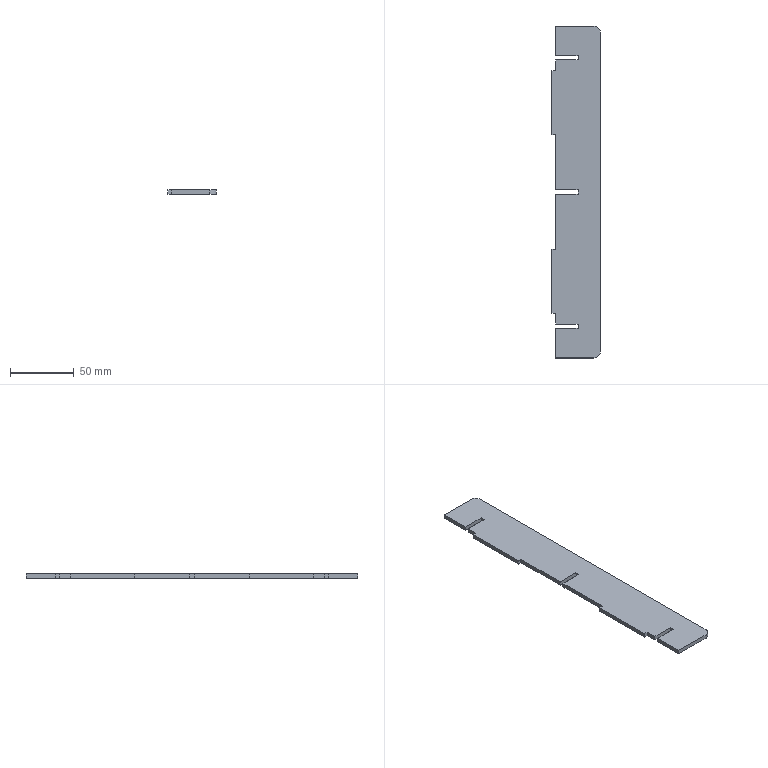Part | SolidWorks | features FlatPattern 1, SMBaseFlange 1, SheetMetal 1 | 1 solid | 28 faces | box 38 x 260 x 3.2 mm | volume 29505 mm3 | plane 26 | cylinder 2 | commonest cylinder face diameters 10 x2
STEP:
#1=CARTESIAN_POINT('',(661.7,-221.227,0.));
#2=VERTEX_POINT('',#1);
#3=CARTESIAN_POINT('',(661.7,-244.627,0.));
#4=VERTEX_POINT('',#3);
#5=CARTESIAN_POINT('',(661.7,-244.627,0.));
#6=DIRECTION('',(0.,-1.,0.));
#7=VECTOR('',#6,1000.);
#8=LINE('',#5,#7);
#9=EDGE_CURVE('',#2,#4,#8,.T.);
#10=ORIENTED_EDGE('',*,*,#9,.F.);
#11=CARTESIAN_POINT('',(661.7,-221.227,-3.2));
#12=VERTEX_POINT('',#11);
#13=CARTESIAN_POINT('',(661.7,-221.227,-3.2));
#14=DIRECTION('',(0.,0.,1.));
#15=VECTOR('',#14,1000.);
#16=LINE('',#13,#15);
#17=EDGE_CURVE('',#12,#2,#16,.T.);
#18=ORIENTED_EDGE('',*,*,#17,.F.);
#19=CARTESIAN_POINT('',(661.7,-244.627,-3.2));
#20=VERTEX_POINT('',#19);
#21=CARTESIAN_POINT('',(661.7,-244.627,-3.2));
#22=DIRECTION('',(0.,-1.,0.));
#23=VECTOR('',#22,1000.);
#24=LINE('',#21,#23);
#25=EDGE_CURVE('',#12,#20,#24,.T.);
#26=ORIENTED_EDGE('',*,*,#25,.T.);
#27=CARTESIAN_POINT('',(661.7,-244.627,-3.2));
#28=DIRECTION('',(0.,0.,1.));
#29=VECTOR('',#28,1000.);
#30=LINE('',#27,#29);
#31=EDGE_CURVE('',#20,#4,#30,.T.);
#32=ORIENTED_EDGE('',*,*,#31,.T.);
#33=EDGE_LOOP('',(#10,#18,#26,#32));
#34=FACE_OUTER_BOUND('',#33,.T.);
#35=CARTESIAN_POINT('',(661.7,-244.627,-3.2));
#36=DIRECTION('',(-1.,0.,0.));
#37=DIRECTION('',(0.,0.,1.));
#38=AXIS2_PLACEMENT_3D('',#35,#36,#37);
#39=PLANE('',#38);
#40=ADVANCED_FACE('',(#34),#39,.T.);
#41=CARTESIAN_POINT('',(679.3,-221.227,0.));
#42=VERTEX_POINT('',#41);
#43=CARTESIAN_POINT('',(661.7,-221.227,0.));
#44=DIRECTION('',(-1.,0.,0.));
#45=VECTOR('',#44,1000.);
#46=LINE('',#43,#45);
#47=EDGE_CURVE('',#42,#2,#46,.T.);
#48=ORIENTED_EDGE('',*,*,#47,.F.);
#49=CARTESIAN_POINT('',(679.3,-221.227,-3.2));
#50=VERTEX_POINT('',#49);
#51=CARTESIAN_POINT('',(679.3,-221.227,-3.2));
#52=DIRECTION('',(0.,0.,1.));
#53=VECTOR('',#52,1000.);
#54=LINE('',#51,#53);
#55=EDGE_CURVE('',#50,#42,#54,.T.);
#56=ORIENTED_EDGE('',*,*,#55,.F.);
#57=CARTESIAN_POINT('',(661.7,-221.227,-3.2));
#58=DIRECTION('',(-1.,0.,0.));
#59=VECTOR('',#58,1000.);
#60=LINE('',#57,#59);
#61=EDGE_CURVE('',#50,#12,#60,.T.);
#62=ORIENTED_EDGE('',*,*,#61,.T.);
#63=ORIENTED_EDGE('',*,*,#17,.T.);
#64=EDGE_LOOP('',(#48,#56,#62,#63));
#65=FACE_OUTER_BOUND('',#64,.T.);
#66=CARTESIAN_POINT('',(661.7,-221.227,-3.2));
#67=DIRECTION('',(0.,1.,0.));
#68=DIRECTION('',(0.,0.,1.));
#69=AXIS2_PLACEMENT_3D('',#66,#67,#68);
#70=PLANE('',#69);
#71=ADVANCED_FACE('',(#65),#70,.T.);
#72=CARTESIAN_POINT('',(679.3,-218.027,0.));
#73=VERTEX_POINT('',#72);
#74=CARTESIAN_POINT('',(679.3,-221.227,0.));
#75=DIRECTION('',(0.,-1.,0.));
#76=VECTOR('',#75,1000.);
#77=LINE('',#74,#76);
#78=EDGE_CURVE('',#73,#42,#77,.T.);
#79=ORIENTED_EDGE('',*,*,#78,.F.);
#80=CARTESIAN_POINT('',(679.3,-218.027,-3.2));
#81=VERTEX_POINT('',#80);
#82=CARTESIAN_POINT('',(679.3,-218.027,-3.2));
#83=DIRECTION('',(0.,0.,1.));
#84=VECTOR('',#83,1000.);
#85=LINE('',#82,#84);
#86=EDGE_CURVE('',#81,#73,#85,.T.);
#87=ORIENTED_EDGE('',*,*,#86,.F.);
#88=CARTESIAN_POINT('',(679.3,-221.227,-3.2));
#89=DIRECTION('',(0.,-1.,0.));
#90=VECTOR('',#89,1000.);
#91=LINE('',#88,#90);
#92=EDGE_CURVE('',#81,#50,#91,.T.);
#93=ORIENTED_EDGE('',*,*,#92,.T.);
#94=ORIENTED_EDGE('',*,*,#55,.T.);
#95=EDGE_LOOP('',(#79,#87,#93,#94));
#96=FACE_OUTER_BOUND('',#95,.T.);
#97=CARTESIAN_POINT('',(679.3,-221.227,-3.2));
#98=DIRECTION('',(-1.,0.,0.));
#99=DIRECTION('',(0.,0.,1.));
#100=AXIS2_PLACEMENT_3D('',#97,#98,#99);
#101=PLANE('',#100);
#102=ADVANCED_FACE('',(#96),#101,.T.);
#103=CARTESIAN_POINT('',(661.7,-218.027,0.));
#104=VERTEX_POINT('',#103);
#105=CARTESIAN_POINT('',(679.3,-218.027,0.));
#106=DIRECTION('',(1.,0.,0.));
#107=VECTOR('',#106,1000.);
#108=LINE('',#105,#107);
#109=EDGE_CURVE('',#104,#73,#108,.T.);
#110=ORIENTED_EDGE('',*,*,#109,.F.);
#111=CARTESIAN_POINT('',(661.7,-218.027,-3.2));
#112=VERTEX_POINT('',#111);
#113=CARTESIAN_POINT('',(661.7,-218.027,-3.2));
#114=DIRECTION('',(0.,0.,1.));
#115=VECTOR('',#114,1000.);
#116=LINE('',#113,#115);
#117=EDGE_CURVE('',#112,#104,#116,.T.);
#118=ORIENTED_EDGE('',*,*,#117,.F.);
#119=CARTESIAN_POINT('',(679.3,-218.027,-3.2));
#120=DIRECTION('',(1.,0.,0.));
#121=VECTOR('',#120,1000.);
#122=LINE('',#119,#121);
#123=EDGE_CURVE('',#112,#81,#122,.T.);
#124=ORIENTED_EDGE('',*,*,#123,.T.);
#125=ORIENTED_EDGE('',*,*,#86,.T.);
#126=EDGE_LOOP('',(#110,#118,#124,#125));
#127=FACE_OUTER_BOUND('',#126,.T.);
#128=CARTESIAN_POINT('',(679.3,-218.027,-3.2));
#129=DIRECTION('',(0.,-1.,0.));
#130=DIRECTION('',(0.,0.,-1.));
#131=AXIS2_PLACEMENT_3D('',#128,#129,#130);
#132=PLANE('',#131);
#133=ADVANCED_FACE('',(#127),#132,.T.);
#134=CARTESIAN_POINT('',(661.7,-209.627,0.));
#135=VERTEX_POINT('',#134);
#136=CARTESIAN_POINT('',(661.7,-218.027,0.));
#137=DIRECTION('',(0.,-1.,0.));
#138=VECTOR('',#137,1000.);
#139=LINE('',#136,#138);
#140=EDGE_CURVE('',#135,#104,#139,.T.);
#141=ORIENTED_EDGE('',*,*,#140,.F.);
#142=CARTESIAN_POINT('',(661.7,-209.627,-3.2));
#143=VERTEX_POINT('',#142);
#144=CARTESIAN_POINT('',(661.7,-209.627,-3.2));
#145=DIRECTION('',(0.,0.,1.));
#146=VECTOR('',#145,1000.);
#147=LINE('',#144,#146);
#148=EDGE_CURVE('',#143,#135,#147,.T.);
#149=ORIENTED_EDGE('',*,*,#148,.F.);
#150=CARTESIAN_POINT('',(661.7,-218.027,-3.2));
#151=DIRECTION('',(0.,-1.,0.));
#152=VECTOR('',#151,1000.);
#153=LINE('',#150,#152);
#154=EDGE_CURVE('',#143,#112,#153,.T.);
#155=ORIENTED_EDGE('',*,*,#154,.T.);
#156=ORIENTED_EDGE('',*,*,#117,.T.);
#157=EDGE_LOOP('',(#141,#149,#155,#156));
#158=FACE_OUTER_BOUND('',#157,.T.);
#159=CARTESIAN_POINT('',(661.7,-218.027,-3.2));
#160=DIRECTION('',(-1.,0.,0.));
#161=DIRECTION('',(0.,0.,1.));
#162=AXIS2_PLACEMENT_3D('',#159,#160,#161);
#163=PLANE('',#162);
#164=ADVANCED_FACE('',(#158),#163,.T.);
#165=CARTESIAN_POINT('',(658.7,-209.627,0.));
#166=VERTEX_POINT('',#165);
#167=CARTESIAN_POINT('',(661.7,-209.627,0.));
#168=DIRECTION('',(1.,0.,0.));
#169=VECTOR('',#168,1000.);
#170=LINE('',#167,#169);
#171=EDGE_CURVE('',#166,#135,#170,.T.);
#172=ORIENTED_EDGE('',*,*,#171,.F.);
#173=CARTESIAN_POINT('',(658.7,-209.627,-3.2));
#174=VERTEX_POINT('',#173);
#175=CARTESIAN_POINT('',(658.7,-209.627,-3.2));
#176=DIRECTION('',(0.,0.,1.));
#177=VECTOR('',#176,1000.);
#178=LINE('',#175,#177);
#179=EDGE_CURVE('',#174,#166,#178,.T.);
#180=ORIENTED_EDGE('',*,*,#179,.F.);
#181=CARTESIAN_POINT('',(661.7,-209.627,-3.2));
#182=DIRECTION('',(1.,0.,0.));
#183=VECTOR('',#182,1000.);
#184=LINE('',#181,#183);
#185=EDGE_CURVE('',#174,#143,#184,.T.);
#186=ORIENTED_EDGE('',*,*,#185,.T.);
#187=ORIENTED_EDGE('',*,*,#148,.T.);
#188=EDGE_LOOP('',(#172,#180,#186,#187));
#189=FACE_OUTER_BOUND('',#188,.T.);
#190=CARTESIAN_POINT('',(661.7,-209.627,-3.2));
#191=DIRECTION('',(0.,-1.,0.));
#192=DIRECTION('',(0.,0.,-1.));
#193=AXIS2_PLACEMENT_3D('',#190,#191,#192);
#194=PLANE('',#193);
#195=ADVANCED_FACE('',(#189),#194,.T.);
#196=CARTESIAN_POINT('',(658.7,-159.627,0.));
#197=VERTEX_POINT('',#196);
#198=CARTESIAN_POINT('',(658.7,-209.627,0.));
#199=DIRECTION('',(0.,-1.,0.));
#200=VECTOR('',#199,1000.);
#201=LINE('',#198,#200);
#202=EDGE_CURVE('',#197,#166,#201,.T.);
#203=ORIENTED_EDGE('',*,*,#202,.F.);
#204=CARTESIAN_POINT('',(658.7,-159.627,-3.2));
#205=VERTEX_POINT('',#204);
#206=CARTESIAN_POINT('',(658.7,-159.627,-3.2));
#207=DIRECTION('',(0.,0.,1.));
#208=VECTOR('',#207,1000.);
#209=LINE('',#206,#208);
#210=EDGE_CURVE('',#205,#197,#209,.T.);
#211=ORIENTED_EDGE('',*,*,#210,.F.);
#212=CARTESIAN_POINT('',(658.7,-209.627,-3.2));
#213=DIRECTION('',(0.,-1.,0.));
#214=VECTOR('',#213,1000.);
#215=LINE('',#212,#214);
#216=EDGE_CURVE('',#205,#174,#215,.T.);
#217=ORIENTED_EDGE('',*,*,#216,.T.);
#218=ORIENTED_EDGE('',*,*,#179,.T.);
#219=EDGE_LOOP('',(#203,#211,#217,#218));
#220=FACE_OUTER_BOUND('',#219,.T.);
#221=CARTESIAN_POINT('',(658.7,-209.627,-3.2));
#222=DIRECTION('',(-1.,0.,0.));
#223=DIRECTION('',(0.,0.,1.));
#224=AXIS2_PLACEMENT_3D('',#221,#222,#223);
#225=PLANE('',#224);
#226=ADVANCED_FACE('',(#220),#225,.T.);
#227=CARTESIAN_POINT('',(661.7,-159.627,0.));
#228=VERTEX_POINT('',#227);
#229=CARTESIAN_POINT('',(658.7,-159.627,0.));
#230=DIRECTION('',(-1.,0.,0.));
#231=VECTOR('',#230,1000.);
#232=LINE('',#229,#231);
#233=EDGE_CURVE('',#228,#197,#232,.T.);
#234=ORIENTED_EDGE('',*,*,#233,.F.);
#235=CARTESIAN_POINT('',(661.7,-159.627,-3.2));
#236=VERTEX_POINT('',#235);
#237=CARTESIAN_POINT('',(661.7,-159.627,-3.2));
#238=DIRECTION('',(0.,0.,1.));
#239=VECTOR('',#238,1000.);
#240=LINE('',#237,#239);
#241=EDGE_CURVE('',#236,#228,#240,.T.);
#242=ORIENTED_EDGE('',*,*,#241,.F.);
#243=CARTESIAN_POINT('',(658.7,-159.627,-3.2));
#244=DIRECTION('',(-1.,0.,0.));
#245=VECTOR('',#244,1000.);
#246=LINE('',#243,#245);
#247=EDGE_CURVE('',#236,#205,#246,.T.);
#248=ORIENTED_EDGE('',*,*,#247,.T.);
#249=ORIENTED_EDGE('',*,*,#210,.T.);
#250=EDGE_LOOP('',(#234,#242,#248,#249));
#251=FACE_OUTER_BOUND('',#250,.T.);
#252=CARTESIAN_POINT('',(658.7,-159.627,-3.2));
#253=DIRECTION('',(0.,1.,0.));
#254=DIRECTION('',(0.,0.,1.));
#255=AXIS2_PLACEMENT_3D('',#252,#253,#254);
#256=PLANE('',#255);
#257=ADVANCED_FACE('',(#251),#256,.T.);
#258=CARTESIAN_POINT('',(661.7,-116.227,0.));
#259=VERTEX_POINT('',#258);
#260=CARTESIAN_POINT('',(661.7,-159.627,0.));
#261=DIRECTION('',(0.,-1.,0.));
#262=VECTOR('',#261,1000.);
#263=LINE('',#260,#262);
#264=EDGE_CURVE('',#259,#228,#263,.T.);
#265=ORIENTED_EDGE('',*,*,#264,.F.);
#266=CARTESIAN_POINT('',(661.7,-116.227,-3.2));
#267=VERTEX_POINT('',#266);
#268=CARTESIAN_POINT('',(661.7,-116.227,-3.2));
#269=DIRECTION('',(0.,0.,1.));
#270=VECTOR('',#269,1000.);
#271=LINE('',#268,#270);
#272=EDGE_CURVE('',#267,#259,#271,.T.);
#273=ORIENTED_EDGE('',*,*,#272,.F.);
#274=CARTESIAN_POINT('',(661.7,-159.627,-3.2));
#275=DIRECTION('',(0.,-1.,0.));
#276=VECTOR('',#275,1000.);
#277=LINE('',#274,#276);
#278=EDGE_CURVE('',#267,#236,#277,.T.);
#279=ORIENTED_EDGE('',*,*,#278,.T.);
#280=ORIENTED_EDGE('',*,*,#241,.T.);
#281=EDGE_LOOP('',(#265,#273,#279,#280));
#282=FACE_OUTER_BOUND('',#281,.T.);
#283=CARTESIAN_POINT('',(661.7,-159.627,-3.2));
#284=DIRECTION('',(-1.,0.,0.));
#285=DIRECTION('',(0.,0.,1.));
#286=AXIS2_PLACEMENT_3D('',#283,#284,#285);
#287=PLANE('',#286);
#288=ADVANCED_FACE('',(#282),#287,.T.);
#289=CARTESIAN_POINT('',(679.3,-116.227,0.));
#290=VERTEX_POINT('',#289);
#291=CARTESIAN_POINT('',(661.7,-116.227,0.));
#292=DIRECTION('',(-1.,0.,0.));
#293=VECTOR('',#292,1000.);
#294=LINE('',#291,#293);
#295=EDGE_CURVE('',#290,#259,#294,.T.);
#296=ORIENTED_EDGE('',*,*,#295,.F.);
#297=CARTESIAN_POINT('',(679.3,-116.227,-3.2));
#298=VERTEX_POINT('',#297);
#299=CARTESIAN_POINT('',(679.3,-116.227,-3.2));
#300=DIRECTION('',(0.,0.,1.));
#301=VECTOR('',#300,1000.);
#302=LINE('',#299,#301);
#303=EDGE_CURVE('',#298,#290,#302,.T.);
#304=ORIENTED_EDGE('',*,*,#303,.F.);
#305=CARTESIAN_POINT('',(661.7,-116.227,-3.2));
#306=DIRECTION('',(-1.,0.,0.));
#307=VECTOR('',#306,1000.);
#308=LINE('',#305,#307);
#309=EDGE_CURVE('',#298,#267,#308,.T.);
#310=ORIENTED_EDGE('',*,*,#309,.T.);
#311=ORIENTED_EDGE('',*,*,#272,.T.);
#312=EDGE_LOOP('',(#296,#304,#310,#311));
#313=FACE_OUTER_BOUND('',#312,.T.);
#314=CARTESIAN_POINT('',(661.7,-116.227,-3.2));
#315=DIRECTION('',(0.,1.,0.));
#316=DIRECTION('',(0.,0.,1.));
#317=AXIS2_PLACEMENT_3D('',#314,#315,#316);
#318=PLANE('',#317);
#319=ADVANCED_FACE('',(#313),#318,.T.);
#320=CARTESIAN_POINT('',(679.3,-113.027,0.));
#321=VERTEX_POINT('',#320);
#322=CARTESIAN_POINT('',(679.3,-116.227,0.));
#323=DIRECTION('',(0.,-1.,0.));
#324=VECTOR('',#323,1000.);
#325=LINE('',#322,#324);
#326=EDGE_CURVE('',#321,#290,#325,.T.);
#327=ORIENTED_EDGE('',*,*,#326,.F.);
#328=CARTESIAN_POINT('',(679.3,-113.027,-3.2));
#329=VERTEX_POINT('',#328);
#330=CARTESIAN_POINT('',(679.3,-113.027,-3.2));
#331=DIRECTION('',(0.,0.,1.));
#332=VECTOR('',#331,1000.);
#333=LINE('',#330,#332);
#334=EDGE_CURVE('',#329,#321,#333,.T.);
#335=ORIENTED_EDGE('',*,*,#334,.F.);
#336=CARTESIAN_POINT('',(679.3,-116.227,-3.2));
#337=DIRECTION('',(0.,-1.,0.));
#338=VECTOR('',#337,1000.);
#339=LINE('',#336,#338);
#340=EDGE_CURVE('',#329,#298,#339,.T.);
#341=ORIENTED_EDGE('',*,*,#340,.T.);
#342=ORIENTED_EDGE('',*,*,#303,.T.);
#343=EDGE_LOOP('',(#327,#335,#341,#342));
#344=FACE_OUTER_BOUND('',#343,.T.);
#345=CARTESIAN_POINT('',(679.3,-116.227,-3.2));
#346=DIRECTION('',(-1.,0.,0.));
#347=DIRECTION('',(0.,0.,1.));
#348=AXIS2_PLACEMENT_3D('',#345,#346,#347);
#349=PLANE('',#348);
#350=ADVANCED_FACE('',(#344),#349,.T.);
#351=CARTESIAN_POINT('',(661.7,-113.027,0.));
#352=VERTEX_POINT('',#351);
#353=CARTESIAN_POINT('',(679.3,-113.027,0.));
#354=DIRECTION('',(1.,0.,0.));
#355=VECTOR('',#354,1000.);
#356=LINE('',#353,#355);
#357=EDGE_CURVE('',#352,#321,#356,.T.);
#358=ORIENTED_EDGE('',*,*,#357,.F.);
#359=CARTESIAN_POINT('',(661.7,-113.027,-3.2));
#360=VERTEX_POINT('',#359);
#361=CARTESIAN_POINT('',(661.7,-113.027,-3.2));
#362=DIRECTION('',(0.,0.,1.));
#363=VECTOR('',#362,1000.);
#364=LINE('',#361,#363);
#365=EDGE_CURVE('',#360,#352,#364,.T.);
#366=ORIENTED_EDGE('',*,*,#365,.F.);
#367=CARTESIAN_POINT('',(679.3,-113.027,-3.2));
#368=DIRECTION('',(1.,0.,0.));
#369=VECTOR('',#368,1000.);
#370=LINE('',#367,#369);
#371=EDGE_CURVE('',#360,#329,#370,.T.);
#372=ORIENTED_EDGE('',*,*,#371,.T.);
#373=ORIENTED_EDGE('',*,*,#334,.T.);
#374=EDGE_LOOP('',(#358,#366,#372,#373));
#375=FACE_OUTER_BOUND('',#374,.T.);
#376=CARTESIAN_POINT('',(679.3,-113.027,-3.2));
#377=DIRECTION('',(0.,-1.,0.));
#378=DIRECTION('',(0.,0.,-1.));
#379=AXIS2_PLACEMENT_3D('',#376,#377,#378);
#380=PLANE('',#379);
#381=ADVANCED_FACE('',(#375),#380,.T.);
#382=CARTESIAN_POINT('',(661.7,-69.627,0.));
#383=VERTEX_POINT('',#382);
#384=CARTESIAN_POINT('',(661.7,-113.027,0.));
#385=DIRECTION('',(0.,-1.,0.));
#386=VECTOR('',#385,1000.);
#387=LINE('',#384,#386);
#388=EDGE_CURVE('',#383,#352,#387,.T.);
#389=ORIENTED_EDGE('',*,*,#388,.F.);
#390=CARTESIAN_POINT('',(661.7,-69.627,-3.2));
#391=VERTEX_POINT('',#390);
#392=CARTESIAN_POINT('',(661.7,-69.627,-3.2));
#393=DIRECTION('',(0.,0.,1.));
#394=VECTOR('',#393,1000.);
#395=LINE('',#392,#394);
#396=EDGE_CURVE('',#391,#383,#395,.T.);
#397=ORIENTED_EDGE('',*,*,#396,.F.);
#398=CARTESIAN_POINT('',(661.7,-113.027,-3.2));
#399=DIRECTION('',(0.,-1.,0.));
#400=VECTOR('',#399,1000.);
#401=LINE('',#398,#400);
#402=EDGE_CURVE('',#391,#360,#401,.T.);
#403=ORIENTED_EDGE('',*,*,#402,.T.);
#404=ORIENTED_EDGE('',*,*,#365,.T.);
#405=EDGE_LOOP('',(#389,#397,#403,#404));
#406=FACE_OUTER_BOUND('',#405,.T.);
#407=CARTESIAN_POINT('',(661.7,-113.027,-3.2));
#408=DIRECTION('',(-1.,0.,0.));
#409=DIRECTION('',(0.,0.,1.));
#410=AXIS2_PLACEMENT_3D('',#407,#408,#409);
#411=PLANE('',#410);
#412=ADVANCED_FACE('',(#406),#411,.T.);
#413=CARTESIAN_POINT('',(658.7,-69.627,0.));
#414=VERTEX_POINT('',#413);
#415=CARTESIAN_POINT('',(658.7,-69.627,0.));
#416=DIRECTION('',(1.,0.,0.));
#417=VECTOR('',#416,1000.);
#418=LINE('',#415,#417);
#419=EDGE_CURVE('',#414,#383,#418,.T.);
#420=ORIENTED_EDGE('',*,*,#419,.F.);
#421=CARTESIAN_POINT('',(658.7,-69.627,-3.2));
#422=VERTEX_POINT('',#421);
#423=CARTESIAN_POINT('',(658.7,-69.627,-3.2));
#424=DIRECTION('',(0.,0.,1.));
#425=VECTOR('',#424,1000.);
#426=LINE('',#423,#425);
#427=EDGE_CURVE('',#422,#414,#426,.T.);
#428=ORIENTED_EDGE('',*,*,#427,.F.);
#429=CARTESIAN_POINT('',(658.7,-69.627,-3.2));
#430=DIRECTION('',(1.,0.,0.));
#431=VECTOR('',#430,1000.);
#432=LINE('',#429,#431);
#433=EDGE_CURVE('',#422,#391,#432,.T.);
#434=ORIENTED_EDGE('',*,*,#433,.T.);
#435=ORIENTED_EDGE('',*,*,#396,.T.);
#436=EDGE_LOOP('',(#420,#428,#434,#435));
#437=FACE_OUTER_BOUND('',#436,.T.);
#438=CARTESIAN_POINT('',(658.7,-69.627,-3.2));
#439=DIRECTION('',(0.,-1.,0.));
#440=DIRECTION('',(0.,0.,-1.));
#441=AXIS2_PLACEMENT_3D('',#438,#439,#440);
#442=PLANE('',#441);
#443=ADVANCED_FACE('',(#437),#442,.T.);
#444=CARTESIAN_POINT('',(658.7,-19.627,0.));
#445=VERTEX_POINT('',#444);
#446=CARTESIAN_POINT('',(658.7,-19.627,0.));
#447=DIRECTION('',(0.,-1.,0.));
#448=VECTOR('',#447,1000.);
#449=LINE('',#446,#448);
#450=EDGE_CURVE('',#445,#414,#449,.T.);
#451=ORIENTED_EDGE('',*,*,#450,.F.);
#452=CARTESIAN_POINT('',(658.7,-19.627,-3.2));
#453=VERTEX_POINT('',#452);
#454=CARTESIAN_POINT('',(658.7,-19.627,-3.2));
#455=DIRECTION('',(0.,0.,1.));
#456=VECTOR('',#455,1000.);
#457=LINE('',#454,#456);
#458=EDGE_CURVE('',#453,#445,#457,.T.);
#459=ORIENTED_EDGE('',*,*,#458,.F.);
#460=CARTESIAN_POINT('',(658.7,-19.627,-3.2));
#461=DIRECTION('',(0.,-1.,0.));
#462=VECTOR('',#461,1000.);
#463=LINE('',#460,#462);
#464=EDGE_CURVE('',#453,#422,#463,.T.);
#465=ORIENTED_EDGE('',*,*,#464,.T.);
#466=ORIENTED_EDGE('',*,*,#427,.T.);
#467=EDGE_LOOP('',(#451,#459,#465,#466));
#468=FACE_OUTER_BOUND('',#467,.T.);
#469=CARTESIAN_POINT('',(658.7,-19.627,-3.2));
#470=DIRECTION('',(-1.,0.,0.));
#471=DIRECTION('',(0.,0.,1.));
#472=AXIS2_PLACEMENT_3D('',#469,#470,#471);
#473=PLANE('',#472);
#474=ADVANCED_FACE('',(#468),#473,.T.);
#475=CARTESIAN_POINT('',(661.7,-19.627,0.));
#476=VERTEX_POINT('',#475);
#477=CARTESIAN_POINT('',(661.7,-19.627,0.));
#478=DIRECTION('',(-1.,0.,0.));
#479=VECTOR('',#478,1000.);
#480=LINE('',#477,#479);
#481=EDGE_CURVE('',#476,#445,#480,.T.);
#482=ORIENTED_EDGE('',*,*,#481,.F.);
#483=CARTESIAN_POINT('',(661.7,-19.627,-3.2));
#484=VERTEX_POINT('',#483);
#485=CARTESIAN_POINT('',(661.7,-19.627,-3.2));
#486=DIRECTION('',(0.,0.,1.));
#487=VECTOR('',#486,1000.);
#488=LINE('',#485,#487);
#489=EDGE_CURVE('',#484,#476,#488,.T.);
#490=ORIENTED_EDGE('',*,*,#489,.F.);
#491=CARTESIAN_POINT('',(661.7,-19.627,-3.2));
#492=DIRECTION('',(-1.,0.,0.));
#493=VECTOR('',#492,1000.);
#494=LINE('',#491,#493);
#495=EDGE_CURVE('',#484,#453,#494,.T.);
#496=ORIENTED_EDGE('',*,*,#495,.T.);
#497=ORIENTED_EDGE('',*,*,#458,.T.);
#498=EDGE_LOOP('',(#482,#490,#496,#497));
#499=FACE_OUTER_BOUND('',#498,.T.);
#500=CARTESIAN_POINT('',(661.7,-19.627,-3.2));
#501=DIRECTION('',(0.,1.,0.));
#502=DIRECTION('',(0.,0.,1.));
#503=AXIS2_PLACEMENT_3D('',#500,#501,#502);
#504=PLANE('',#503);
#505=ADVANCED_FACE('',(#499),#504,.T.);
#506=CARTESIAN_POINT('',(661.7,-11.227,0.));
#507=VERTEX_POINT('',#506);
#508=CARTESIAN_POINT('',(661.7,-19.627,0.));
#509=DIRECTION('',(0.,-1.,0.));
#510=VECTOR('',#509,1000.);
#511=LINE('',#508,#510);
#512=EDGE_CURVE('',#507,#476,#511,.T.);
#513=ORIENTED_EDGE('',*,*,#512,.F.);
#514=CARTESIAN_POINT('',(661.7,-11.227,-3.2));
#515=VERTEX_POINT('',#514);
#516=CARTESIAN_POINT('',(661.7,-11.227,-3.2));
#517=DIRECTION('',(0.,0.,1.));
#518=VECTOR('',#517,1000.);
#519=LINE('',#516,#518);
#520=EDGE_CURVE('',#515,#507,#519,.T.);
#521=ORIENTED_EDGE('',*,*,#520,.F.);
#522=CARTESIAN_POINT('',(661.7,-19.627,-3.2));
#523=DIRECTION('',(0.,-1.,0.));
#524=VECTOR('',#523,1000.);
#525=LINE('',#522,#524);
#526=EDGE_CURVE('',#515,#484,#525,.T.);
#527=ORIENTED_EDGE('',*,*,#526,.T.);
#528=ORIENTED_EDGE('',*,*,#489,.T.);
#529=EDGE_LOOP('',(#513,#521,#527,#528));
#530=FACE_OUTER_BOUND('',#529,.T.);
#531=CARTESIAN_POINT('',(661.7,-19.627,-3.2));
#532=DIRECTION('',(-1.,0.,0.));
#533=DIRECTION('',(0.,0.,1.));
#534=AXIS2_PLACEMENT_3D('',#531,#532,#533);
#535=PLANE('',#534);
#536=ADVANCED_FACE('',(#530),#535,.T.);
#537=CARTESIAN_POINT('',(679.3,-11.227,0.));
#538=VERTEX_POINT('',#537);
#539=CARTESIAN_POINT('',(661.7,-11.227,0.));
#540=DIRECTION('',(-1.,0.,0.));
#541=VECTOR('',#540,1000.);
#542=LINE('',#539,#541);
#543=EDGE_CURVE('',#538,#507,#542,.T.);
#544=ORIENTED_EDGE('',*,*,#543,.F.);
#545=CARTESIAN_POINT('',(679.3,-11.227,-3.2));
#546=VERTEX_POINT('',#545);
#547=CARTESIAN_POINT('',(679.3,-11.227,-3.2));
#548=DIRECTION('',(0.,0.,1.));
#549=VECTOR('',#548,1000.);
#550=LINE('',#547,#549);
#551=EDGE_CURVE('',#546,#538,#550,.T.);
#552=ORIENTED_EDGE('',*,*,#551,.F.);
#553=CARTESIAN_POINT('',(661.7,-11.227,-3.2));
#554=DIRECTION('',(-1.,0.,0.));
#555=VECTOR('',#554,1000.);
#556=LINE('',#553,#555);
#557=EDGE_CURVE('',#546,#515,#556,.T.);
#558=ORIENTED_EDGE('',*,*,#557,.T.);
#559=ORIENTED_EDGE('',*,*,#520,.T.);
#560=EDGE_LOOP('',(#544,#552,#558,#559));
#561=FACE_OUTER_BOUND('',#560,.T.);
#562=CARTESIAN_POINT('',(661.7,-11.227,-3.2));
#563=DIRECTION('',(0.,1.,0.));
#564=DIRECTION('',(0.,0.,1.));
#565=AXIS2_PLACEMENT_3D('',#562,#563,#564);
#566=PLANE('',#565);
#567=ADVANCED_FACE('',(#561),#566,.T.);
#568=CARTESIAN_POINT('',(679.3,-8.027,0.));
#569=VERTEX_POINT('',#568);
#570=CARTESIAN_POINT('',(679.3,-11.227,0.));
#571=DIRECTION('',(0.,-1.,0.));
#572=VECTOR('',#571,1000.);
#573=LINE('',#570,#572);
#574=EDGE_CURVE('',#569,#538,#573,.T.);
#575=ORIENTED_EDGE('',*,*,#574,.F.);
#576=CARTESIAN_POINT('',(679.3,-8.027,-3.2));
#577=VERTEX_POINT('',#576);
#578=CARTESIAN_POINT('',(679.3,-8.027,-3.2));
#579=DIRECTION('',(0.,0.,1.));
#580=VECTOR('',#579,1000.);
#581=LINE('',#578,#580);
#582=EDGE_CURVE('',#577,#569,#581,.T.);
#583=ORIENTED_EDGE('',*,*,#582,.F.);
#584=CARTESIAN_POINT('',(679.3,-11.227,-3.2));
#585=DIRECTION('',(0.,-1.,0.));
#586=VECTOR('',#585,1000.);
#587=LINE('',#584,#586);
#588=EDGE_CURVE('',#577,#546,#587,.T.);
#589=ORIENTED_EDGE('',*,*,#588,.T.);
#590=ORIENTED_EDGE('',*,*,#551,.T.);
#591=EDGE_LOOP('',(#575,#583,#589,#590));
#592=FACE_OUTER_BOUND('',#591,.T.);
#593=CARTESIAN_POINT('',(679.3,-11.227,-3.2));
#594=DIRECTION('',(-1.,0.,0.));
#595=DIRECTION('',(0.,0.,1.));
#596=AXIS2_PLACEMENT_3D('',#593,#594,#595);
#597=PLANE('',#596);
#598=ADVANCED_FACE('',(#592),#597,.T.);
#599=CARTESIAN_POINT('',(661.7,-8.027,0.));
#600=VERTEX_POINT('',#599);
#601=CARTESIAN_POINT('',(679.3,-8.027,0.));
#602=DIRECTION('',(1.,0.,0.));
#603=VECTOR('',#602,1000.);
#604=LINE('',#601,#603);
#605=EDGE_CURVE('',#600,#569,#604,.T.);
#606=ORIENTED_EDGE('',*,*,#605,.F.);
#607=CARTESIAN_POINT('',(661.7,-8.027,-3.2));
#608=VERTEX_POINT('',#607);
#609=CARTESIAN_POINT('',(661.7,-8.027,-3.2));
#610=DIRECTION('',(0.,0.,1.));
#611=VECTOR('',#610,1000.);
#612=LINE('',#609,#611);
#613=EDGE_CURVE('',#608,#600,#612,.T.);
#614=ORIENTED_EDGE('',*,*,#613,.F.);
#615=CARTESIAN_POINT('',(679.3,-8.027,-3.2));
#616=DIRECTION('',(1.,0.,0.));
#617=VECTOR('',#616,1000.);
#618=LINE('',#615,#617);
#619=EDGE_CURVE('',#608,#577,#618,.T.);
#620=ORIENTED_EDGE('',*,*,#619,.T.);
#621=ORIENTED_EDGE('',*,*,#582,.T.);
#622=EDGE_LOOP('',(#606,#614,#620,#621));
#623=FACE_OUTER_BOUND('',#622,.T.);
#624=CARTESIAN_POINT('',(679.3,-8.027,-3.2));
#625=DIRECTION('',(0.,-1.,0.));
#626=DIRECTION('',(0.,0.,-1.));
#627=AXIS2_PLACEMENT_3D('',#624,#625,#626);
#628=PLANE('',#627);
#629=ADVANCED_FACE('',(#623),#628,.T.);
#630=CARTESIAN_POINT('',(661.7,15.373,0.));
#631=VERTEX_POINT('',#630);
#632=CARTESIAN_POINT('',(661.7,-8.027,0.));
#633=DIRECTION('',(0.,-1.,0.));
#634=VECTOR('',#633,1000.);
#635=LINE('',#632,#634);
#636=EDGE_CURVE('',#631,#600,#635,.T.);
#637=ORIENTED_EDGE('',*,*,#636,.F.);
#638=CARTESIAN_POINT('',(661.7,15.373,-3.2));
#639=VERTEX_POINT('',#638);
#640=CARTESIAN_POINT('',(661.7,15.373,-3.2));
#641=DIRECTION('',(0.,0.,1.));
#642=VECTOR('',#641,1000.);
#643=LINE('',#640,#642);
#644=EDGE_CURVE('',#639,#631,#643,.T.);
#645=ORIENTED_EDGE('',*,*,#644,.F.);
#646=CARTESIAN_POINT('',(661.7,-8.027,-3.2));
#647=DIRECTION('',(0.,-1.,0.));
#648=VECTOR('',#647,1000.);
#649=LINE('',#646,#648);
#650=EDGE_CURVE('',#639,#608,#649,.T.);
#651=ORIENTED_EDGE('',*,*,#650,.T.);
#652=ORIENTED_EDGE('',*,*,#613,.T.);
#653=EDGE_LOOP('',(#637,#645,#651,#652));
#654=FACE_OUTER_BOUND('',#653,.T.);
#655=CARTESIAN_POINT('',(661.7,-8.027,-3.2));
#656=DIRECTION('',(-1.,0.,0.));
#657=DIRECTION('',(0.,0.,1.));
#658=AXIS2_PLACEMENT_3D('',#655,#656,#657);
#659=PLANE('',#658);
#660=ADVANCED_FACE('',(#654),#659,.T.);
#661=CARTESIAN_POINT('',(691.7,15.373,0.));
#662=VERTEX_POINT('',#661);
#663=CARTESIAN_POINT('',(661.7,15.373,0.));
#664=DIRECTION('',(-1.,0.,0.));
#665=VECTOR('',#664,1000.);
#666=LINE('',#663,#665);
#667=EDGE_CURVE('',#662,#631,#666,.T.);
#668=ORIENTED_EDGE('',*,*,#667,.F.);
#669=CARTESIAN_POINT('',(691.7,15.373,-3.2));
#670=VERTEX_POINT('',#669);
#671=CARTESIAN_POINT('',(691.7,15.373,-3.2));
#672=DIRECTION('',(0.,0.,1.));
#673=VECTOR('',#672,1000.);
#674=LINE('',#671,#673);
#675=EDGE_CURVE('',#670,#662,#674,.T.);
#676=ORIENTED_EDGE('',*,*,#675,.F.);
#677=CARTESIAN_POINT('',(661.7,15.373,-3.2));
#678=DIRECTION('',(-1.,0.,0.));
#679=VECTOR('',#678,1000.);
#680=LINE('',#677,#679);
#681=EDGE_CURVE('',#670,#639,#680,.T.);
#682=ORIENTED_EDGE('',*,*,#681,.T.);
#683=ORIENTED_EDGE('',*,*,#644,.T.);
#684=EDGE_LOOP('',(#668,#676,#682,#683));
#685=FACE_OUTER_BOUND('',#684,.T.);
#686=CARTESIAN_POINT('',(661.7,15.373,-3.2));
#687=DIRECTION('',(0.,1.,0.));
#688=DIRECTION('',(0.,0.,1.));
#689=AXIS2_PLACEMENT_3D('',#686,#687,#688);
#690=PLANE('',#689);
#691=ADVANCED_FACE('',(#685),#690,.T.);
#692=CARTESIAN_POINT('',(696.7,10.373,0.));
#693=VERTEX_POINT('',#692);
#694=CARTESIAN_POINT('',(691.7,10.373,0.));
#695=DIRECTION('',(0.,0.,1.));
#696=DIRECTION('',(-1.,0.,0.));
#697=AXIS2_PLACEMENT_3D('',#694,#695,#696);
#698=CIRCLE('',#697,5.);
#699=EDGE_CURVE('',#693,#662,#698,.T.);
#700=ORIENTED_EDGE('',*,*,#699,.F.);
#701=CARTESIAN_POINT('',(696.7,10.373,-3.2));
#702=VERTEX_POINT('',#701);
#703=CARTESIAN_POINT('',(696.7,10.373,-3.2));
#704=DIRECTION('',(0.,0.,1.));
#705=VECTOR('',#704,1000.);
#706=LINE('',#703,#705);
#707=EDGE_CURVE('',#702,#693,#706,.T.);
#708=ORIENTED_EDGE('',*,*,#707,.F.);
#709=CARTESIAN_POINT('',(691.7,10.373,-3.2));
#710=DIRECTION('',(0.,0.,1.));
#711=DIRECTION('',(-1.,0.,0.));
#712=AXIS2_PLACEMENT_3D('',#709,#710,#711);
#713=CIRCLE('',#712,5.);
#714=EDGE_CURVE('',#702,#670,#713,.T.);
#715=ORIENTED_EDGE('',*,*,#714,.T.);
#716=ORIENTED_EDGE('',*,*,#675,.T.);
#717=EDGE_LOOP('',(#700,#708,#715,#716));
#718=FACE_OUTER_BOUND('',#717,.T.);
#719=CARTESIAN_POINT('',(691.7,10.373,-3.2));
#720=DIRECTION('',(0.,0.,1.));
#721=DIRECTION('',(1.,0.,0.));
#722=AXIS2_PLACEMENT_3D('',#719,#720,#721);
#723=CYLINDRICAL_SURFACE('',#722,5.);
#724=ADVANCED_FACE('',(#718),#723,.T.);
#725=CARTESIAN_POINT('',(696.7,-239.627,0.));
#726=VERTEX_POINT('',#725);
#727=CARTESIAN_POINT('',(696.7,-239.627,0.));
#728=DIRECTION('',(0.,1.,0.));
#729=VECTOR('',#728,1000.);
#730=LINE('',#727,#729);
#731=EDGE_CURVE('',#726,#693,#730,.T.);
#732=ORIENTED_EDGE('',*,*,#731,.F.);
#733=CARTESIAN_POINT('',(696.7,-239.627,-3.2));
#734=VERTEX_POINT('',#733);
#735=CARTESIAN_POINT('',(696.7,-239.627,-3.2));
#736=DIRECTION('',(0.,0.,1.));
#737=VECTOR('',#736,1000.);
#738=LINE('',#735,#737);
#739=EDGE_CURVE('',#734,#726,#738,.T.);
#740=ORIENTED_EDGE('',*,*,#739,.F.);
#741=CARTESIAN_POINT('',(696.7,-239.627,-3.2));
#742=DIRECTION('',(0.,1.,0.));
#743=VECTOR('',#742,1000.);
#744=LINE('',#741,#743);
#745=EDGE_CURVE('',#734,#702,#744,.T.);
#746=ORIENTED_EDGE('',*,*,#745,.T.);
#747=ORIENTED_EDGE('',*,*,#707,.T.);
#748=EDGE_LOOP('',(#732,#740,#746,#747));
#749=FACE_OUTER_BOUND('',#748,.T.);
#750=CARTESIAN_POINT('',(696.7,-239.627,-3.2));
#751=DIRECTION('',(1.,0.,0.));
#752=DIRECTION('',(0.,0.,-1.));
#753=AXIS2_PLACEMENT_3D('',#750,#751,#752);
#754=PLANE('',#753);
#755=ADVANCED_FACE('',(#749),#754,.T.);
#756=CARTESIAN_POINT('',(691.7,-244.627,0.));
#757=VERTEX_POINT('',#756);
#758=CARTESIAN_POINT('',(691.7,-239.627,0.));
#759=DIRECTION('',(0.,0.,1.));
#760=DIRECTION('',(1.,0.,0.));
#761=AXIS2_PLACEMENT_3D('',#758,#759,#760);
#762=CIRCLE('',#761,5.);
#763=EDGE_CURVE('',#757,#726,#762,.T.);
#764=ORIENTED_EDGE('',*,*,#763,.F.);
#765=CARTESIAN_POINT('',(691.7,-244.627,-3.2));
#766=VERTEX_POINT('',#765);
#767=CARTESIAN_POINT('',(691.7,-244.627,-3.2));
#768=DIRECTION('',(0.,0.,1.));
#769=VECTOR('',#768,1000.);
#770=LINE('',#767,#769);
#771=EDGE_CURVE('',#766,#757,#770,.T.);
#772=ORIENTED_EDGE('',*,*,#771,.F.);
#773=CARTESIAN_POINT('',(691.7,-239.627,-3.2));
#774=DIRECTION('',(0.,0.,1.));
#775=DIRECTION('',(1.,0.,0.));
#776=AXIS2_PLACEMENT_3D('',#773,#774,#775);
#777=CIRCLE('',#776,5.);
#778=EDGE_CURVE('',#766,#734,#777,.T.);
#779=ORIENTED_EDGE('',*,*,#778,.T.);
#780=ORIENTED_EDGE('',*,*,#739,.T.);
#781=EDGE_LOOP('',(#764,#772,#779,#780));
#782=FACE_OUTER_BOUND('',#781,.T.);
#783=CARTESIAN_POINT('',(691.7,-239.627,-3.2));
#784=DIRECTION('',(0.,0.,1.));
#785=DIRECTION('',(1.,0.,0.));
#786=AXIS2_PLACEMENT_3D('',#783,#784,#785);
#787=CYLINDRICAL_SURFACE('',#786,5.);
#788=ADVANCED_FACE('',(#782),#787,.T.);
#789=CARTESIAN_POINT('',(661.7,-244.627,0.));
#790=DIRECTION('',(1.,0.,0.));
#791=VECTOR('',#790,1000.);
#792=LINE('',#789,#791);
#793=EDGE_CURVE('',#4,#757,#792,.T.);
#794=ORIENTED_EDGE('',*,*,#793,.F.);
#795=ORIENTED_EDGE('',*,*,#31,.F.);
#796=CARTESIAN_POINT('',(661.7,-244.627,-3.2));
#797=DIRECTION('',(1.,0.,0.));
#798=VECTOR('',#797,1000.);
#799=LINE('',#796,#798);
#800=EDGE_CURVE('',#20,#766,#799,.T.);
#801=ORIENTED_EDGE('',*,*,#800,.T.);
#802=ORIENTED_EDGE('',*,*,#771,.T.);
#803=EDGE_LOOP('',(#794,#795,#801,#802));
#804=FACE_OUTER_BOUND('',#803,.T.);
#805=CARTESIAN_POINT('',(661.7,-244.627,-3.2));
#806=DIRECTION('',(0.,-1.,0.));
#807=DIRECTION('',(0.,0.,-1.));
#808=AXIS2_PLACEMENT_3D('',#805,#806,#807);
#809=PLANE('',#808);
#810=ADVANCED_FACE('',(#804),#809,.T.);
#811=ORIENTED_EDGE('',*,*,#25,.F.);
#812=ORIENTED_EDGE('',*,*,#61,.F.);
#813=ORIENTED_EDGE('',*,*,#92,.F.);
#814=ORIENTED_EDGE('',*,*,#123,.F.);
#815=ORIENTED_EDGE('',*,*,#154,.F.);
#816=ORIENTED_EDGE('',*,*,#185,.F.);
#817=ORIENTED_EDGE('',*,*,#216,.F.);
#818=ORIENTED_EDGE('',*,*,#247,.F.);
#819=ORIENTED_EDGE('',*,*,#278,.F.);
#820=ORIENTED_EDGE('',*,*,#309,.F.);
#821=ORIENTED_EDGE('',*,*,#340,.F.);
#822=ORIENTED_EDGE('',*,*,#371,.F.);
#823=ORIENTED_EDGE('',*,*,#402,.F.);
#824=ORIENTED_EDGE('',*,*,#433,.F.);
#825=ORIENTED_EDGE('',*,*,#464,.F.);
#826=ORIENTED_EDGE('',*,*,#495,.F.);
#827=ORIENTED_EDGE('',*,*,#526,.F.);
#828=ORIENTED_EDGE('',*,*,#557,.F.);
#829=ORIENTED_EDGE('',*,*,#588,.F.);
#830=ORIENTED_EDGE('',*,*,#619,.F.);
#831=ORIENTED_EDGE('',*,*,#650,.F.);
#832=ORIENTED_EDGE('',*,*,#681,.F.);
#833=ORIENTED_EDGE('',*,*,#714,.F.);
#834=ORIENTED_EDGE('',*,*,#745,.F.);
#835=ORIENTED_EDGE('',*,*,#778,.F.);
#836=ORIENTED_EDGE('',*,*,#800,.F.);
#837=EDGE_LOOP('',(#811,#812,#813,#814,#815,#816,#817,#818,#819,#820,#821,#822,#823,#824,#825,#826,#827,#828,#829,#830,#831,#832,#833,#834,#835,#836));
#838=FACE_OUTER_BOUND('',#837,.T.);
#839=CARTESIAN_POINT('',(691.7,10.373,-3.2));
#840=DIRECTION('',(0.,0.,-1.));
#841=DIRECTION('',(-1.,0.,0.));
#842=AXIS2_PLACEMENT_3D('',#839,#840,#841);
#843=PLANE('',#842);
#844=ADVANCED_FACE('',(#838),#843,.T.);
#845=ORIENTED_EDGE('',*,*,#9,.T.);
#846=ORIENTED_EDGE('',*,*,#793,.T.);
#847=ORIENTED_EDGE('',*,*,#763,.T.);
#848=ORIENTED_EDGE('',*,*,#731,.T.);
#849=ORIENTED_EDGE('',*,*,#699,.T.);
#850=ORIENTED_EDGE('',*,*,#667,.T.);
#851=ORIENTED_EDGE('',*,*,#636,.T.);
#852=ORIENTED_EDGE('',*,*,#605,.T.);
#853=ORIENTED_EDGE('',*,*,#574,.T.);
#854=ORIENTED_EDGE('',*,*,#543,.T.);
#855=ORIENTED_EDGE('',*,*,#512,.T.);
#856=ORIENTED_EDGE('',*,*,#481,.T.);
#857=ORIENTED_EDGE('',*,*,#450,.T.);
#858=ORIENTED_EDGE('',*,*,#419,.T.);
#859=ORIENTED_EDGE('',*,*,#388,.T.);
#860=ORIENTED_EDGE('',*,*,#357,.T.);
#861=ORIENTED_EDGE('',*,*,#326,.T.);
#862=ORIENTED_EDGE('',*,*,#295,.T.);
#863=ORIENTED_EDGE('',*,*,#264,.T.);
#864=ORIENTED_EDGE('',*,*,#233,.T.);
#865=ORIENTED_EDGE('',*,*,#202,.T.);
#866=ORIENTED_EDGE('',*,*,#171,.T.);
#867=ORIENTED_EDGE('',*,*,#140,.T.);
#868=ORIENTED_EDGE('',*,*,#109,.T.);
#869=ORIENTED_EDGE('',*,*,#78,.T.);
#870=ORIENTED_EDGE('',*,*,#47,.T.);
#871=EDGE_LOOP('',(#845,#846,#847,#848,#849,#850,#851,#852,#853,#854,#855,#856,#857,#858,#859,#860,#861,#862,#863,#864,#865,#866,#867,#868,#869,#870));
#872=FACE_OUTER_BOUND('',#871,.T.);
#873=CARTESIAN_POINT('',(691.7,10.373,0.));
#874=DIRECTION('',(0.,0.,-1.));
#875=DIRECTION('',(-1.,0.,0.));
#876=AXIS2_PLACEMENT_3D('',#873,#874,#875);
#877=PLANE('',#876);
#878=ADVANCED_FACE('',(#872),#877,.F.);
#879=CLOSED_SHELL('',(#40,#71,#102,#133,#164,#195,#226,#257,#288,#319,#350,#381,#412,#443,#474,#505,#536,#567,#598,#629,#660,#691,#724,#755,#788,#810,#844,#878));
#880=MANIFOLD_SOLID_BREP('',#879);
#881=CARTESIAN_POINT('',(0.,0.,0.));
#882=DIRECTION('',(0.,0.,1.));
#883=DIRECTION('',(1.,0.,0.));
#884=AXIS2_PLACEMENT_3D('',#881,#882,#883);
#885=(LENGTH_UNIT()NAMED_UNIT(*)SI_UNIT(.MILLI.,.METRE.));
#886=UNCERTAINTY_MEASURE_WITH_UNIT(LENGTH_MEASURE(0.00001),#885,'','');
#887=(NAMED_UNIT(*)PLANE_ANGLE_UNIT()SI_UNIT($,.RADIAN.));
#888=(NAMED_UNIT(*)SI_UNIT($,.STERADIAN.)SOLID_ANGLE_UNIT());
#889=(GEOMETRIC_REPRESENTATION_CONTEXT(3)GLOBAL_UNCERTAINTY_ASSIGNED_CONTEXT((#886))GLOBAL_UNIT_ASSIGNED_CONTEXT((#885,#887,#888))REPRESENTATION_CONTEXT('',''));
#890=ADVANCED_BREP_SHAPE_REPRESENTATION('',(#880,#884),#889);